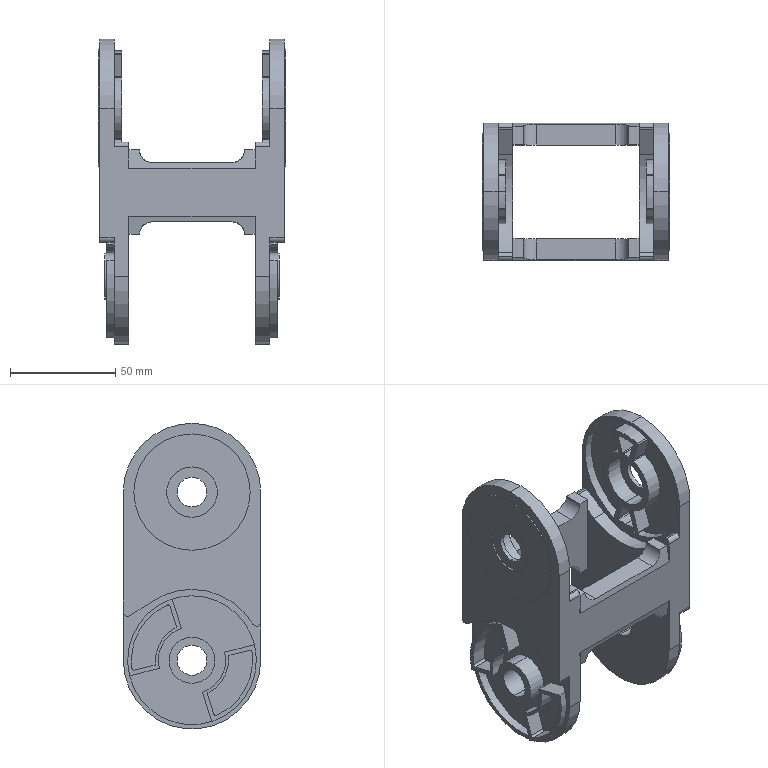Part | SolidWorks | features BaseBody 1 | 1 solid | 262 faces | box 89 x 65.39 x 145.39 mm | volume 145575 mm3 | cylinder 160 | plane 102 | commonest cylinder face diameters 1 x44 2 x12 4 x12 61.27 x10 24 x8 30.68 x6